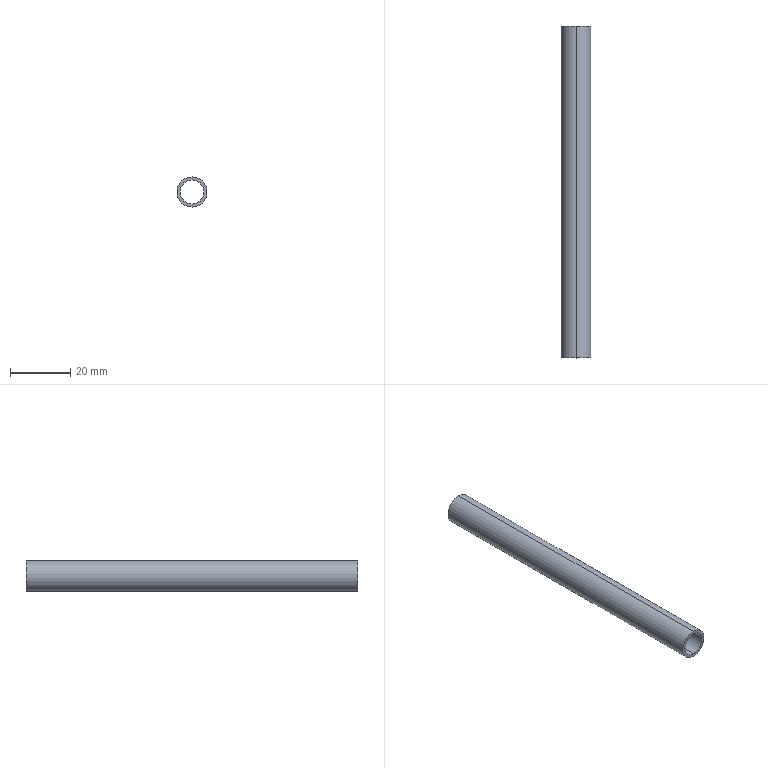Part | SolidWorks | features Sweep 1 | 1 solid | 6 faces | box 10 x 110 x 10 mm | volume 3110 mm3 | cylinder 4 | plane 2 | commonest cylinder face diameters 8 x2 10 x2
STEP:
#1=CARTESIAN_POINT('',(0.,0.,4.));
#2=VERTEX_POINT('',#1);
#3=CARTESIAN_POINT('',(0.,0.,-4.));
#4=VERTEX_POINT('',#3);
#5=CARTESIAN_POINT('',(0.,0.,0.));
#6=DIRECTION('',(0.,-1.,0.));
#7=DIRECTION('',(0.,0.,1.));
#8=AXIS2_PLACEMENT_3D('',#5,#6,#7);
#9=CIRCLE('',#8,4.);
#10=EDGE_CURVE('',#2,#4,#9,.T.);
#11=ORIENTED_EDGE('',*,*,#10,.T.);
#12=CARTESIAN_POINT('',(0.,110.,-4.));
#13=VERTEX_POINT('',#12);
#14=CARTESIAN_POINT('',(0.,0.,-4.));
#15=DIRECTION('',(0.,1.,0.));
#16=VECTOR('',#15,1000.);
#17=LINE('',#14,#16);
#18=EDGE_CURVE('',#4,#13,#17,.T.);
#19=ORIENTED_EDGE('',*,*,#18,.T.);
#20=CARTESIAN_POINT('',(0.,110.,4.));
#21=VERTEX_POINT('',#20);
#22=CARTESIAN_POINT('',(0.,110.,0.));
#23=DIRECTION('',(0.,-1.,0.));
#24=DIRECTION('',(0.,0.,1.));
#25=AXIS2_PLACEMENT_3D('',#22,#23,#24);
#26=CIRCLE('',#25,4.);
#27=EDGE_CURVE('',#21,#13,#26,.T.);
#28=ORIENTED_EDGE('',*,*,#27,.F.);
#29=CARTESIAN_POINT('',(0.,0.,4.));
#30=DIRECTION('',(0.,1.,0.));
#31=VECTOR('',#30,1000.);
#32=LINE('',#29,#31);
#33=EDGE_CURVE('',#2,#21,#32,.T.);
#34=ORIENTED_EDGE('',*,*,#33,.F.);
#35=EDGE_LOOP('',(#11,#19,#28,#34));
#36=FACE_OUTER_BOUND('',#35,.T.);
#37=CARTESIAN_POINT('',(0.,0.,0.));
#38=DIRECTION('',(0.,1.,0.));
#39=DIRECTION('',(0.,0.,1.));
#40=AXIS2_PLACEMENT_3D('',#37,#38,#39);
#41=CYLINDRICAL_SURFACE('',#40,4.);
#42=ADVANCED_FACE('',(#36),#41,.F.);
#43=CARTESIAN_POINT('',(0.,0.,5.));
#44=VERTEX_POINT('',#43);
#45=CARTESIAN_POINT('',(0.,0.,-5.));
#46=VERTEX_POINT('',#45);
#47=CARTESIAN_POINT('',(0.,0.,0.));
#48=DIRECTION('',(0.,1.,0.));
#49=DIRECTION('',(0.,0.,1.));
#50=AXIS2_PLACEMENT_3D('',#47,#48,#49);
#51=CIRCLE('',#50,5.);
#52=EDGE_CURVE('',#44,#46,#51,.T.);
#53=ORIENTED_EDGE('',*,*,#52,.T.);
#54=CARTESIAN_POINT('',(0.,110.,-5.));
#55=VERTEX_POINT('',#54);
#56=CARTESIAN_POINT('',(0.,0.,-5.));
#57=DIRECTION('',(0.,1.,0.));
#58=VECTOR('',#57,1000.);
#59=LINE('',#56,#58);
#60=EDGE_CURVE('',#46,#55,#59,.T.);
#61=ORIENTED_EDGE('',*,*,#60,.T.);
#62=CARTESIAN_POINT('',(0.,110.,5.));
#63=VERTEX_POINT('',#62);
#64=CARTESIAN_POINT('',(0.,110.,0.));
#65=DIRECTION('',(0.,1.,0.));
#66=DIRECTION('',(0.,0.,1.));
#67=AXIS2_PLACEMENT_3D('',#64,#65,#66);
#68=CIRCLE('',#67,5.);
#69=EDGE_CURVE('',#63,#55,#68,.T.);
#70=ORIENTED_EDGE('',*,*,#69,.F.);
#71=CARTESIAN_POINT('',(0.,0.,5.));
#72=DIRECTION('',(0.,1.,0.));
#73=VECTOR('',#72,1000.);
#74=LINE('',#71,#73);
#75=EDGE_CURVE('',#44,#63,#74,.T.);
#76=ORIENTED_EDGE('',*,*,#75,.F.);
#77=EDGE_LOOP('',(#53,#61,#70,#76));
#78=FACE_OUTER_BOUND('',#77,.T.);
#79=CARTESIAN_POINT('',(0.,0.,0.));
#80=DIRECTION('',(0.,1.,0.));
#81=DIRECTION('',(0.,0.,1.));
#82=AXIS2_PLACEMENT_3D('',#79,#80,#81);
#83=CYLINDRICAL_SURFACE('',#82,5.);
#84=ADVANCED_FACE('',(#78),#83,.T.);
#85=ORIENTED_EDGE('',*,*,#18,.F.);
#86=CARTESIAN_POINT('',(0.,0.,0.));
#87=DIRECTION('',(0.,-1.,0.));
#88=DIRECTION('',(0.,0.,1.));
#89=AXIS2_PLACEMENT_3D('',#86,#87,#88);
#90=CIRCLE('',#89,4.);
#91=EDGE_CURVE('',#4,#2,#90,.T.);
#92=ORIENTED_EDGE('',*,*,#91,.T.);
#93=ORIENTED_EDGE('',*,*,#33,.T.);
#94=CARTESIAN_POINT('',(0.,110.,0.));
#95=DIRECTION('',(0.,-1.,0.));
#96=DIRECTION('',(0.,0.,1.));
#97=AXIS2_PLACEMENT_3D('',#94,#95,#96);
#98=CIRCLE('',#97,4.);
#99=EDGE_CURVE('',#13,#21,#98,.T.);
#100=ORIENTED_EDGE('',*,*,#99,.F.);
#101=EDGE_LOOP('',(#85,#92,#93,#100));
#102=FACE_OUTER_BOUND('',#101,.T.);
#103=CARTESIAN_POINT('',(0.,0.,0.));
#104=DIRECTION('',(0.,1.,0.));
#105=DIRECTION('',(0.,0.,1.));
#106=AXIS2_PLACEMENT_3D('',#103,#104,#105);
#107=CYLINDRICAL_SURFACE('',#106,4.);
#108=ADVANCED_FACE('',(#102),#107,.F.);
#109=ORIENTED_EDGE('',*,*,#27,.T.);
#110=ORIENTED_EDGE('',*,*,#99,.T.);
#111=EDGE_LOOP('',(#109,#110));
#112=FACE_BOUND('',#111,.T.);
#113=ORIENTED_EDGE('',*,*,#69,.T.);
#114=CARTESIAN_POINT('',(0.,110.,0.));
#115=DIRECTION('',(0.,1.,0.));
#116=DIRECTION('',(0.,0.,1.));
#117=AXIS2_PLACEMENT_3D('',#114,#115,#116);
#118=CIRCLE('',#117,5.);
#119=EDGE_CURVE('',#55,#63,#118,.T.);
#120=ORIENTED_EDGE('',*,*,#119,.T.);
#121=EDGE_LOOP('',(#113,#120));
#122=FACE_OUTER_BOUND('',#121,.T.);
#123=CARTESIAN_POINT('',(0.,110.,0.));
#124=DIRECTION('',(0.,1.,0.));
#125=DIRECTION('',(0.,0.,1.));
#126=AXIS2_PLACEMENT_3D('',#123,#124,#125);
#127=PLANE('',#126);
#128=ADVANCED_FACE('',(#112,#122),#127,.T.);
#129=ORIENTED_EDGE('',*,*,#10,.F.);
#130=ORIENTED_EDGE('',*,*,#91,.F.);
#131=EDGE_LOOP('',(#129,#130));
#132=FACE_BOUND('',#131,.T.);
#133=ORIENTED_EDGE('',*,*,#52,.F.);
#134=CARTESIAN_POINT('',(0.,0.,0.));
#135=DIRECTION('',(0.,1.,0.));
#136=DIRECTION('',(0.,0.,1.));
#137=AXIS2_PLACEMENT_3D('',#134,#135,#136);
#138=CIRCLE('',#137,5.);
#139=EDGE_CURVE('',#46,#44,#138,.T.);
#140=ORIENTED_EDGE('',*,*,#139,.F.);
#141=EDGE_LOOP('',(#133,#140));
#142=FACE_OUTER_BOUND('',#141,.T.);
#143=CARTESIAN_POINT('',(0.,0.,0.));
#144=DIRECTION('',(0.,1.,0.));
#145=DIRECTION('',(0.,0.,1.));
#146=AXIS2_PLACEMENT_3D('',#143,#144,#145);
#147=PLANE('',#146);
#148=ADVANCED_FACE('',(#132,#142),#147,.F.);
#149=ORIENTED_EDGE('',*,*,#60,.F.);
#150=ORIENTED_EDGE('',*,*,#139,.T.);
#151=ORIENTED_EDGE('',*,*,#75,.T.);
#152=ORIENTED_EDGE('',*,*,#119,.F.);
#153=EDGE_LOOP('',(#149,#150,#151,#152));
#154=FACE_OUTER_BOUND('',#153,.T.);
#155=CARTESIAN_POINT('',(0.,0.,0.));
#156=DIRECTION('',(0.,1.,0.));
#157=DIRECTION('',(0.,0.,1.));
#158=AXIS2_PLACEMENT_3D('',#155,#156,#157);
#159=CYLINDRICAL_SURFACE('',#158,5.);
#160=ADVANCED_FACE('',(#154),#159,.T.);
#161=CLOSED_SHELL('',(#42,#84,#108,#128,#148,#160));
#162=MANIFOLD_SOLID_BREP('',#161);
#163=CARTESIAN_POINT('',(0.,0.,0.));
#164=DIRECTION('',(0.,0.,1.));
#165=DIRECTION('',(1.,0.,0.));
#166=AXIS2_PLACEMENT_3D('',#163,#164,#165);
#167=(LENGTH_UNIT()NAMED_UNIT(*)SI_UNIT(.MILLI.,.METRE.));
#168=UNCERTAINTY_MEASURE_WITH_UNIT(LENGTH_MEASURE(0.00001),#167,'','');
#169=(NAMED_UNIT(*)PLANE_ANGLE_UNIT()SI_UNIT($,.RADIAN.));
#170=(NAMED_UNIT(*)SI_UNIT($,.STERADIAN.)SOLID_ANGLE_UNIT());
#171=(GEOMETRIC_REPRESENTATION_CONTEXT(3)GLOBAL_UNCERTAINTY_ASSIGNED_CONTEXT((#168))GLOBAL_UNIT_ASSIGNED_CONTEXT((#167,#169,#170))REPRESENTATION_CONTEXT('',''));
#172=ADVANCED_BREP_SHAPE_REPRESENTATION('',(#162,#166),#171);